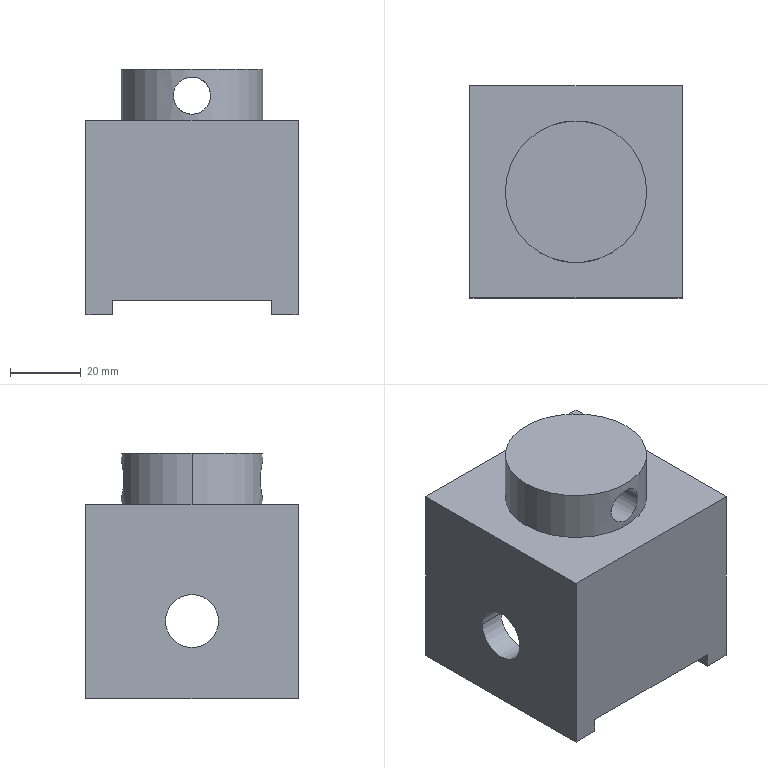Part | NX | features BREP 1 | 1 solid | 23 faces | box 60 x 60 x 69.5 mm | volume 83417 mm3 | plane 15 | cylinder 8 | commonest cylinder face diameters 15 x4 10.5 x2 40 x2
STEP:
#1=CARTESIAN_POINT('',(-5.25,-19.299,7.));
#2=VERTEX_POINT('',#1);
#3=CARTESIAN_POINT('',(5.25,-19.299,7.));
#4=VERTEX_POINT('',#3);
#5=CARTESIAN_POINT('',(-5.25,-19.299,7.));
#6=CARTESIAN_POINT('',(-5.25,-19.299,6.68));
#7=CARTESIAN_POINT('',(-5.203,-19.312,6.178));
#8=CARTESIAN_POINT('',(-5.05,-19.353,5.525));
#9=CARTESIAN_POINT('',(-4.847,-19.404,4.964));
#10=CARTESIAN_POINT('',(-4.714,-19.437,4.682));
#11=CARTESIAN_POINT('',(-4.41,-19.511,4.109));
#12=CARTESIAN_POINT('',(-3.746,-19.654,3.244));
#13=CARTESIAN_POINT('',(-2.935,-19.786,2.621));
#14=CARTESIAN_POINT('',(-2.357,-19.86,2.304));
#15=CARTESIAN_POINT('',(-2.046,-19.896,2.157));
#16=CARTESIAN_POINT('',(-1.491,-19.946,1.955));
#17=CARTESIAN_POINT('',(-0.8306,-19.986,1.798));
#18=CARTESIAN_POINT('',(-0.005315,-20.008,1.718));
#19=CARTESIAN_POINT('',(0.8212,-19.987,1.797));
#20=CARTESIAN_POINT('',(1.478,-19.947,1.951));
#21=CARTESIAN_POINT('',(2.033,-19.898,2.152));
#22=CARTESIAN_POINT('',(2.33,-19.864,2.291));
#23=CARTESIAN_POINT('',(2.909,-19.79,2.605));
#24=CARTESIAN_POINT('',(3.547,-19.687,3.081));
#25=CARTESIAN_POINT('',(4.166,-19.564,3.784));
#26=CARTESIAN_POINT('',(4.479,-19.495,4.243));
#27=CARTESIAN_POINT('',(4.716,-19.437,4.684));
#28=CARTESIAN_POINT('',(4.84,-19.406,4.949));
#29=CARTESIAN_POINT('',(5.049,-19.353,5.522));
#30=CARTESIAN_POINT('',(5.202,-19.312,6.177));
#31=CARTESIAN_POINT('',(5.25,-19.299,6.681));
#32=CARTESIAN_POINT('',(5.25,-19.299,7.));
#33=B_SPLINE_CURVE_WITH_KNOTS('',3,(#5,#6,#7,#8,#9,#10,#11,#12,#13,#14,#15,#16,#17,#18,#19,#20,#21,#22,#23,#24,#25,#26,#27,#28,#29,#30,#31,#32),.UNSPECIFIED.,.F.,.F.,(4,1,1,1,1,1,1,1,1,1,1,1,1,1,1,1,1,1,1,1,1,1,1,1,1,4),(0.,0.0625,0.09375,0.125,0.1562,0.1875,0.25,0.3125,0.3438,0.375,0.4062,0.4375,0.5,0.5625,0.5938,0.625,0.6562,0.6875,0.75,0.7812,0.8125,0.8438,0.875,0.9062,0.9375,1.),.UNSPECIFIED.);
#34=EDGE_CURVE('',#2,#4,#33,.T.);
#35=ORIENTED_EDGE('',*,*,#34,.T.);
#36=CARTESIAN_POINT('',(5.25,19.299,7.));
#37=VERTEX_POINT('',#36);
#38=CARTESIAN_POINT('',(5.25,-19.299,7.));
#39=DIRECTION('',(0.,1.,0.));
#40=VECTOR('',#39,1000.);
#41=LINE('',#38,#40);
#42=EDGE_CURVE('',#37,#4,#41,.F.);
#43=ORIENTED_EDGE('',*,*,#42,.F.);
#44=CARTESIAN_POINT('',(-5.25,19.299,7.));
#45=VERTEX_POINT('',#44);
#46=CARTESIAN_POINT('',(5.25,19.299,7.));
#47=CARTESIAN_POINT('',(5.25,19.299,6.678));
#48=CARTESIAN_POINT('',(5.202,19.313,6.172));
#49=CARTESIAN_POINT('',(5.047,19.354,5.514));
#50=CARTESIAN_POINT('',(4.837,19.406,4.943));
#51=CARTESIAN_POINT('',(4.71,19.439,4.671));
#52=CARTESIAN_POINT('',(4.47,19.497,4.229));
#53=CARTESIAN_POINT('',(4.156,19.566,3.771));
#54=CARTESIAN_POINT('',(3.535,19.69,3.07));
#55=CARTESIAN_POINT('',(2.903,19.791,2.601));
#56=CARTESIAN_POINT('',(2.323,19.865,2.287));
#57=CARTESIAN_POINT('',(2.019,19.9,2.147));
#58=CARTESIAN_POINT('',(1.469,19.948,1.949));
#59=CARTESIAN_POINT('',(0.8131,19.987,1.796));
#60=CARTESIAN_POINT('',(-0.01179,20.009,1.718));
#61=CARTESIAN_POINT('',(-0.8396,19.986,1.8));
#62=CARTESIAN_POINT('',(-1.496,19.946,1.957));
#63=CARTESIAN_POINT('',(-2.051,19.896,2.16));
#64=CARTESIAN_POINT('',(-2.347,19.862,2.299));
#65=CARTESIAN_POINT('',(-2.921,19.788,2.611));
#66=CARTESIAN_POINT('',(-3.746,19.654,3.242));
#67=CARTESIAN_POINT('',(-4.407,19.512,4.104));
#68=CARTESIAN_POINT('',(-4.711,19.438,4.676));
#69=CARTESIAN_POINT('',(-4.842,19.405,4.953));
#70=CARTESIAN_POINT('',(-5.048,19.353,5.518));
#71=CARTESIAN_POINT('',(-5.202,19.312,6.174));
#72=CARTESIAN_POINT('',(-5.25,19.299,6.679));
#73=CARTESIAN_POINT('',(-5.25,19.299,7.));
#74=B_SPLINE_CURVE_WITH_KNOTS('',3,(#46,#47,#48,#49,#50,#51,#52,#53,#54,#55,#56,#57,#58,#59,#60,#61,#62,#63,#64,#65,#66,#67,#68,#69,#70,#71,#72,#73),.UNSPECIFIED.,.F.,.F.,(4,1,1,1,1,1,1,1,1,1,1,1,1,1,1,1,1,1,1,1,1,1,1,1,1,4),(0.,0.0625,0.09375,0.125,0.1562,0.1875,0.2188,0.25,0.3125,0.3438,0.375,0.4062,0.4375,0.5,0.5625,0.5938,0.625,0.6562,0.6875,0.75,0.8125,0.8438,0.875,0.9062,0.9375,1.),.UNSPECIFIED.);
#75=EDGE_CURVE('',#45,#37,#74,.F.);
#76=ORIENTED_EDGE('',*,*,#75,.F.);
#77=CARTESIAN_POINT('',(-5.25,-19.299,7.));
#78=DIRECTION('',(0.,1.,0.));
#79=VECTOR('',#78,1000.);
#80=LINE('',#77,#79);
#81=EDGE_CURVE('',#45,#2,#80,.F.);
#82=ORIENTED_EDGE('',*,*,#81,.T.);
#83=EDGE_LOOP('',(#35,#43,#76,#82));
#84=FACE_BOUND('',#83,.T.);
#85=CARTESIAN_POINT('',(0.,0.,7.));
#86=DIRECTION('',(0.,1.,0.));
#87=DIRECTION('',(-1.,0.,0.));
#88=AXIS2_PLACEMENT_3D('',#85,#86,#87);
#89=CYLINDRICAL_SURFACE('',#88,5.25);
#90=ADVANCED_FACE('',(#84),#89,.F.);
#91=CARTESIAN_POINT('',(5.25,-19.299,7.));
#92=CARTESIAN_POINT('',(5.25,-19.299,7.313));
#93=CARTESIAN_POINT('',(5.204,-19.312,7.811));
#94=CARTESIAN_POINT('',(5.052,-19.353,8.467));
#95=CARTESIAN_POINT('',(4.847,-19.405,9.036));
#96=CARTESIAN_POINT('',(4.712,-19.438,9.323));
#97=CARTESIAN_POINT('',(4.405,-19.512,9.899));
#98=CARTESIAN_POINT('',(3.748,-19.653,10.754));
#99=CARTESIAN_POINT('',(2.936,-19.786,11.379));
#100=CARTESIAN_POINT('',(2.358,-19.86,11.695));
#101=CARTESIAN_POINT('',(2.046,-19.896,11.842));
#102=CARTESIAN_POINT('',(1.494,-19.946,12.044));
#103=CARTESIAN_POINT('',(0.8342,-19.986,12.201));
#104=CARTESIAN_POINT('',(0.006992,-20.009,12.282));
#105=CARTESIAN_POINT('',(-0.8194,-19.987,12.203));
#106=CARTESIAN_POINT('',(-1.476,-19.947,12.049));
#107=CARTESIAN_POINT('',(-2.03,-19.898,11.849));
#108=CARTESIAN_POINT('',(-2.33,-19.863,11.71));
#109=CARTESIAN_POINT('',(-2.91,-19.789,11.394));
#110=CARTESIAN_POINT('',(-3.544,-19.688,10.922));
#111=CARTESIAN_POINT('',(-4.169,-19.563,10.212));
#112=CARTESIAN_POINT('',(-4.482,-19.494,9.752));
#113=CARTESIAN_POINT('',(-4.718,-19.437,9.312));
#114=CARTESIAN_POINT('',(-4.839,-19.406,9.053));
#115=CARTESIAN_POINT('',(-5.049,-19.353,8.48));
#116=CARTESIAN_POINT('',(-5.202,-19.312,7.825));
#117=CARTESIAN_POINT('',(-5.25,-19.299,7.32));
#118=CARTESIAN_POINT('',(-5.25,-19.299,7.));
#119=B_SPLINE_CURVE_WITH_KNOTS('',3,(#91,#92,#93,#94,#95,#96,#97,#98,#99,#100,#101,#102,#103,#104,#105,#106,#107,#108,#109,#110,#111,#112,#113,#114,#115,#116,#117,#118),.UNSPECIFIED.,.F.,.F.,(4,1,1,1,1,1,1,1,1,1,1,1,1,1,1,1,1,1,1,1,1,1,1,1,1,4),(0.,0.0625,0.09375,0.125,0.1562,0.1875,0.25,0.3125,0.3438,0.375,0.4062,0.4375,0.5,0.5625,0.5938,0.625,0.6562,0.6875,0.75,0.7812,0.8125,0.8438,0.875,0.9062,0.9375,1.),.UNSPECIFIED.);
#120=EDGE_CURVE('',#4,#2,#119,.T.);
#121=ORIENTED_EDGE('',*,*,#120,.T.);
#122=ORIENTED_EDGE('',*,*,#81,.F.);
#123=CARTESIAN_POINT('',(-5.25,19.299,7.));
#124=CARTESIAN_POINT('',(-5.25,19.299,7.322));
#125=CARTESIAN_POINT('',(-5.202,19.313,7.828));
#126=CARTESIAN_POINT('',(-5.047,19.354,8.487));
#127=CARTESIAN_POINT('',(-4.838,19.406,9.057));
#128=CARTESIAN_POINT('',(-4.709,19.439,9.33));
#129=CARTESIAN_POINT('',(-4.469,19.497,9.773));
#130=CARTESIAN_POINT('',(-4.154,19.566,10.232));
#131=CARTESIAN_POINT('',(-3.533,19.69,10.931));
#132=CARTESIAN_POINT('',(-2.898,19.792,11.402));
#133=CARTESIAN_POINT('',(-2.316,19.866,11.717));
#134=CARTESIAN_POINT('',(-2.007,19.901,11.858));
#135=CARTESIAN_POINT('',(-1.458,19.949,12.055));
#136=CARTESIAN_POINT('',(-0.8011,19.988,12.206));
#137=CARTESIAN_POINT('',(0.02533,20.009,12.282));
#138=CARTESIAN_POINT('',(0.8493,19.986,12.198));
#139=CARTESIAN_POINT('',(1.504,19.946,12.041));
#140=CARTESIAN_POINT('',(2.057,19.896,11.838));
#141=CARTESIAN_POINT('',(2.353,19.861,11.698));
#142=CARTESIAN_POINT('',(2.925,19.788,11.386));
#143=CARTESIAN_POINT('',(3.75,19.653,10.753));
#144=CARTESIAN_POINT('',(4.408,19.512,9.894));
#145=CARTESIAN_POINT('',(4.713,19.438,9.321));
#146=CARTESIAN_POINT('',(4.844,19.405,9.041));
#147=CARTESIAN_POINT('',(5.05,19.353,8.475));
#148=CARTESIAN_POINT('',(5.203,19.312,7.821));
#149=CARTESIAN_POINT('',(5.25,19.299,7.318));
#150=CARTESIAN_POINT('',(5.25,19.299,7.));
#151=B_SPLINE_CURVE_WITH_KNOTS('',3,(#123,#124,#125,#126,#127,#128,#129,#130,#131,#132,#133,#134,#135,#136,#137,#138,#139,#140,#141,#142,#143,#144,#145,#146,#147,#148,#149,#150),.UNSPECIFIED.,.F.,.F.,(4,1,1,1,1,1,1,1,1,1,1,1,1,1,1,1,1,1,1,1,1,1,1,1,1,4),(0.,0.0625,0.09375,0.125,0.1562,0.1875,0.2188,0.25,0.3125,0.3438,0.375,0.4062,0.4375,0.5,0.5625,0.5938,0.625,0.6562,0.6875,0.75,0.8125,0.8438,0.875,0.9062,0.9375,1.),.UNSPECIFIED.);
#152=EDGE_CURVE('',#37,#45,#151,.F.);
#153=ORIENTED_EDGE('',*,*,#152,.F.);
#154=ORIENTED_EDGE('',*,*,#42,.T.);
#155=EDGE_LOOP('',(#121,#122,#153,#154));
#156=FACE_BOUND('',#155,.T.);
#157=CARTESIAN_POINT('',(0.,0.,7.));
#158=DIRECTION('',(0.,1.,0.));
#159=DIRECTION('',(-1.,0.,0.));
#160=AXIS2_PLACEMENT_3D('',#157,#158,#159);
#161=CYLINDRICAL_SURFACE('',#160,5.25);
#162=ADVANCED_FACE('',(#156),#161,.F.);
#163=CARTESIAN_POINT('',(-20.,0.,0.));
#164=VERTEX_POINT('',#163);
#165=CARTESIAN_POINT('',(20.,0.,0.));
#166=VERTEX_POINT('',#165);
#167=CARTESIAN_POINT('',(0.,0.,0.));
#168=DIRECTION('',(0.,0.,-1.));
#169=DIRECTION('',(-1.,0.,0.));
#170=AXIS2_PLACEMENT_3D('',#167,#168,#169);
#171=CIRCLE('',#170,20.);
#172=EDGE_CURVE('',#164,#166,#171,.T.);
#173=ORIENTED_EDGE('',*,*,#172,.F.);
#174=CARTESIAN_POINT('',(-20.,0.,14.5));
#175=VERTEX_POINT('',#174);
#176=CARTESIAN_POINT('',(-20.,0.,14.5));
#177=DIRECTION('',(0.,0.,-1.));
#178=VECTOR('',#177,1000.);
#179=LINE('',#176,#178);
#180=EDGE_CURVE('',#175,#164,#179,.T.);
#181=ORIENTED_EDGE('',*,*,#180,.F.);
#182=CARTESIAN_POINT('',(20.,0.,14.5));
#183=VERTEX_POINT('',#182);
#184=CARTESIAN_POINT('',(0.,0.,14.5));
#185=DIRECTION('',(0.,0.,1.));
#186=DIRECTION('',(1.,0.,0.));
#187=AXIS2_PLACEMENT_3D('',#184,#185,#186);
#188=CIRCLE('',#187,20.);
#189=EDGE_CURVE('',#183,#175,#188,.T.);
#190=ORIENTED_EDGE('',*,*,#189,.F.);
#191=CARTESIAN_POINT('',(20.,0.,14.5));
#192=DIRECTION('',(0.,0.,-1.));
#193=VECTOR('',#192,1000.);
#194=LINE('',#191,#193);
#195=EDGE_CURVE('',#183,#166,#194,.T.);
#196=ORIENTED_EDGE('',*,*,#195,.T.);
#197=EDGE_LOOP('',(#173,#181,#190,#196));
#198=FACE_BOUND('',#197,.T.);
#199=ORIENTED_EDGE('',*,*,#75,.T.);
#200=ORIENTED_EDGE('',*,*,#152,.T.);
#201=EDGE_LOOP('',(#199,#200));
#202=FACE_BOUND('',#201,.T.);
#203=CARTESIAN_POINT('',(0.,0.,7.25));
#204=DIRECTION('',(0.,0.,1.));
#205=DIRECTION('',(1.,0.,0.));
#206=AXIS2_PLACEMENT_3D('',#203,#204,#205);
#207=CYLINDRICAL_SURFACE('',#206,20.);
#208=ADVANCED_FACE('',(#198,#202),#207,.T.);
#209=CARTESIAN_POINT('',(0.,0.,0.));
#210=DIRECTION('',(0.,0.,-1.));
#211=DIRECTION('',(1.,0.,0.));
#212=AXIS2_PLACEMENT_3D('',#209,#210,#211);
#213=CIRCLE('',#212,20.);
#214=EDGE_CURVE('',#166,#164,#213,.T.);
#215=ORIENTED_EDGE('',*,*,#214,.F.);
#216=ORIENTED_EDGE('',*,*,#195,.F.);
#217=CARTESIAN_POINT('',(0.,0.,14.5));
#218=DIRECTION('',(0.,0.,1.));
#219=DIRECTION('',(-1.,0.,0.));
#220=AXIS2_PLACEMENT_3D('',#217,#218,#219);
#221=CIRCLE('',#220,20.);
#222=EDGE_CURVE('',#175,#183,#221,.T.);
#223=ORIENTED_EDGE('',*,*,#222,.F.);
#224=ORIENTED_EDGE('',*,*,#180,.T.);
#225=EDGE_LOOP('',(#215,#216,#223,#224));
#226=FACE_BOUND('',#225,.T.);
#227=ORIENTED_EDGE('',*,*,#120,.F.);
#228=ORIENTED_EDGE('',*,*,#34,.F.);
#229=EDGE_LOOP('',(#227,#228));
#230=FACE_BOUND('',#229,.T.);
#231=CARTESIAN_POINT('',(0.,0.,7.25));
#232=DIRECTION('',(0.,0.,1.));
#233=DIRECTION('',(1.,0.,0.));
#234=AXIS2_PLACEMENT_3D('',#231,#232,#233);
#235=CYLINDRICAL_SURFACE('',#234,20.);
#236=ADVANCED_FACE('',(#226,#230),#235,.T.);
#237=ORIENTED_EDGE('',*,*,#222,.T.);
#238=ORIENTED_EDGE('',*,*,#189,.T.);
#239=EDGE_LOOP('',(#237,#238));
#240=FACE_BOUND('',#239,.T.);
#241=CARTESIAN_POINT('',(0.,0.,14.5));
#242=DIRECTION('',(0.,0.,1.));
#243=DIRECTION('',(1.,0.,0.));
#244=AXIS2_PLACEMENT_3D('',#241,#242,#243);
#245=PLANE('',#244);
#246=ADVANCED_FACE('',(#240),#245,.T.);
#247=CARTESIAN_POINT('',(30.,-30.,0.));
#248=VERTEX_POINT('',#247);
#249=CARTESIAN_POINT('',(-30.,-30.,0.));
#250=VERTEX_POINT('',#249);
#251=CARTESIAN_POINT('',(30.,-30.,0.));
#252=DIRECTION('',(-1.,0.,0.));
#253=VECTOR('',#252,1000.);
#254=LINE('',#251,#253);
#255=EDGE_CURVE('',#248,#250,#254,.T.);
#256=ORIENTED_EDGE('',*,*,#255,.F.);
#257=CARTESIAN_POINT('',(30.,30.,0.));
#258=VERTEX_POINT('',#257);
#259=CARTESIAN_POINT('',(30.,30.,0.));
#260=DIRECTION('',(0.,-1.,0.));
#261=VECTOR('',#260,1000.);
#262=LINE('',#259,#261);
#263=EDGE_CURVE('',#258,#248,#262,.T.);
#264=ORIENTED_EDGE('',*,*,#263,.F.);
#265=CARTESIAN_POINT('',(-30.,30.,0.));
#266=VERTEX_POINT('',#265);
#267=CARTESIAN_POINT('',(30.,30.,0.));
#268=DIRECTION('',(-1.,0.,0.));
#269=VECTOR('',#268,1000.);
#270=LINE('',#267,#269);
#271=EDGE_CURVE('',#258,#266,#270,.T.);
#272=ORIENTED_EDGE('',*,*,#271,.T.);
#273=CARTESIAN_POINT('',(-30.,30.,0.));
#274=DIRECTION('',(0.,-1.,0.));
#275=VECTOR('',#274,1000.);
#276=LINE('',#273,#275);
#277=EDGE_CURVE('',#266,#250,#276,.T.);
#278=ORIENTED_EDGE('',*,*,#277,.T.);
#279=EDGE_LOOP('',(#256,#264,#272,#278));
#280=FACE_BOUND('',#279,.T.);
#281=ORIENTED_EDGE('',*,*,#172,.T.);
#282=ORIENTED_EDGE('',*,*,#214,.T.);
#283=EDGE_LOOP('',(#281,#282));
#284=FACE_BOUND('',#283,.T.);
#285=CARTESIAN_POINT('',(30.,0.,0.));
#286=DIRECTION('',(0.,0.,-1.));
#287=DIRECTION('',(0.,-1.,0.));
#288=AXIS2_PLACEMENT_3D('',#285,#286,#287);
#289=PLANE('',#288);
#290=ADVANCED_FACE('',(#280,#284),#289,.F.);
#291=CARTESIAN_POINT('',(-30.,-30.,-55.));
#292=VERTEX_POINT('',#291);
#293=CARTESIAN_POINT('',(-30.,-30.,0.));
#294=DIRECTION('',(0.,0.,-1.));
#295=VECTOR('',#294,1000.);
#296=LINE('',#293,#295);
#297=EDGE_CURVE('',#250,#292,#296,.T.);
#298=ORIENTED_EDGE('',*,*,#297,.F.);
#299=ORIENTED_EDGE('',*,*,#277,.F.);
#300=CARTESIAN_POINT('',(-30.,30.,-55.));
#301=VERTEX_POINT('',#300);
#302=CARTESIAN_POINT('',(-30.,30.,0.));
#303=DIRECTION('',(0.,0.,-1.));
#304=VECTOR('',#303,1000.);
#305=LINE('',#302,#304);
#306=EDGE_CURVE('',#266,#301,#305,.T.);
#307=ORIENTED_EDGE('',*,*,#306,.T.);
#308=CARTESIAN_POINT('',(-30.,30.,-55.));
#309=DIRECTION('',(0.,-1.,0.));
#310=VECTOR('',#309,1000.);
#311=LINE('',#308,#310);
#312=EDGE_CURVE('',#301,#292,#311,.T.);
#313=ORIENTED_EDGE('',*,*,#312,.T.);
#314=EDGE_LOOP('',(#298,#299,#307,#313));
#315=FACE_BOUND('',#314,.T.);
#316=CARTESIAN_POINT('',(-30.,-7.5,-33.));
#317=VERTEX_POINT('',#316);
#318=CARTESIAN_POINT('',(-30.,7.5,-33.));
#319=VERTEX_POINT('',#318);
#320=CARTESIAN_POINT('',(-30.,0.,-33.));
#321=DIRECTION('',(1.,0.,0.));
#322=DIRECTION('',(0.,-1.,0.));
#323=AXIS2_PLACEMENT_3D('',#320,#321,#322);
#324=CIRCLE('',#323,7.5);
#325=EDGE_CURVE('',#317,#319,#324,.T.);
#326=ORIENTED_EDGE('',*,*,#325,.T.);
#327=CARTESIAN_POINT('',(-30.,0.,-33.));
#328=DIRECTION('',(1.,0.,0.));
#329=DIRECTION('',(0.,1.,0.));
#330=AXIS2_PLACEMENT_3D('',#327,#328,#329);
#331=CIRCLE('',#330,7.5);
#332=EDGE_CURVE('',#319,#317,#331,.T.);
#333=ORIENTED_EDGE('',*,*,#332,.T.);
#334=EDGE_LOOP('',(#326,#333));
#335=FACE_BOUND('',#334,.T.);
#336=CARTESIAN_POINT('',(-30.,0.,-55.));
#337=DIRECTION('',(-1.,0.,0.));
#338=DIRECTION('',(0.,0.,1.));
#339=AXIS2_PLACEMENT_3D('',#336,#337,#338);
#340=PLANE('',#339);
#341=ADVANCED_FACE('',(#315,#335),#340,.T.);
#342=CARTESIAN_POINT('',(22.5,30.,-55.));
#343=VERTEX_POINT('',#342);
#344=CARTESIAN_POINT('',(30.,30.,-55.));
#345=VERTEX_POINT('',#344);
#346=CARTESIAN_POINT('',(22.5,30.,-55.));
#347=DIRECTION('',(1.,0.,0.));
#348=VECTOR('',#347,1000.);
#349=LINE('',#346,#348);
#350=EDGE_CURVE('',#343,#345,#349,.T.);
#351=ORIENTED_EDGE('',*,*,#350,.T.);
#352=CARTESIAN_POINT('',(30.,-30.,-55.));
#353=VERTEX_POINT('',#352);
#354=CARTESIAN_POINT('',(30.,30.,-55.));
#355=DIRECTION('',(0.,-1.,0.));
#356=VECTOR('',#355,1000.);
#357=LINE('',#354,#356);
#358=EDGE_CURVE('',#345,#353,#357,.T.);
#359=ORIENTED_EDGE('',*,*,#358,.T.);
#360=CARTESIAN_POINT('',(22.5,-30.,-55.));
#361=VERTEX_POINT('',#360);
#362=CARTESIAN_POINT('',(22.5,-30.,-55.));
#363=DIRECTION('',(1.,0.,0.));
#364=VECTOR('',#363,1000.);
#365=LINE('',#362,#364);
#366=EDGE_CURVE('',#361,#353,#365,.T.);
#367=ORIENTED_EDGE('',*,*,#366,.F.);
#368=CARTESIAN_POINT('',(22.5,-30.,-55.));
#369=DIRECTION('',(0.,1.,0.));
#370=VECTOR('',#369,1000.);
#371=LINE('',#368,#370);
#372=EDGE_CURVE('',#361,#343,#371,.T.);
#373=ORIENTED_EDGE('',*,*,#372,.T.);
#374=EDGE_LOOP('',(#351,#359,#367,#373));
#375=FACE_BOUND('',#374,.T.);
#376=CARTESIAN_POINT('',(22.5,0.,-55.));
#377=DIRECTION('',(0.,0.,1.));
#378=DIRECTION('',(1.,0.,0.));
#379=AXIS2_PLACEMENT_3D('',#376,#377,#378);
#380=PLANE('',#379);
#381=ADVANCED_FACE('',(#375),#380,.F.);
#382=CARTESIAN_POINT('',(-22.5,-30.,-55.));
#383=VERTEX_POINT('',#382);
#384=CARTESIAN_POINT('',(-30.,-30.,-55.));
#385=DIRECTION('',(1.,0.,0.));
#386=VECTOR('',#385,1000.);
#387=LINE('',#384,#386);
#388=EDGE_CURVE('',#292,#383,#387,.T.);
#389=ORIENTED_EDGE('',*,*,#388,.F.);
#390=ORIENTED_EDGE('',*,*,#312,.F.);
#391=CARTESIAN_POINT('',(-22.5,30.,-55.));
#392=VERTEX_POINT('',#391);
#393=CARTESIAN_POINT('',(-30.,30.,-55.));
#394=DIRECTION('',(1.,0.,0.));
#395=VECTOR('',#394,1000.);
#396=LINE('',#393,#395);
#397=EDGE_CURVE('',#301,#392,#396,.T.);
#398=ORIENTED_EDGE('',*,*,#397,.T.);
#399=CARTESIAN_POINT('',(-22.5,30.,-55.));
#400=DIRECTION('',(0.,-1.,0.));
#401=VECTOR('',#400,1000.);
#402=LINE('',#399,#401);
#403=EDGE_CURVE('',#392,#383,#402,.T.);
#404=ORIENTED_EDGE('',*,*,#403,.T.);
#405=EDGE_LOOP('',(#389,#390,#398,#404));
#406=FACE_BOUND('',#405,.T.);
#407=CARTESIAN_POINT('',(22.5,0.,-55.));
#408=DIRECTION('',(0.,0.,1.));
#409=DIRECTION('',(1.,0.,0.));
#410=AXIS2_PLACEMENT_3D('',#407,#408,#409);
#411=PLANE('',#410);
#412=ADVANCED_FACE('',(#406),#411,.F.);
#413=CARTESIAN_POINT('',(22.5,28.,-5.));
#414=VERTEX_POINT('',#413);
#415=CARTESIAN_POINT('',(22.5,-28.,-5.));
#416=VERTEX_POINT('',#415);
#417=CARTESIAN_POINT('',(22.5,28.,-5.));
#418=DIRECTION('',(0.,-1.,0.));
#419=VECTOR('',#418,1000.);
#420=LINE('',#417,#419);
#421=EDGE_CURVE('',#414,#416,#420,.T.);
#422=ORIENTED_EDGE('',*,*,#421,.F.);
#423=CARTESIAN_POINT('',(22.5,28.,-51.));
#424=VERTEX_POINT('',#423);
#425=CARTESIAN_POINT('',(22.5,28.,-51.));
#426=DIRECTION('',(0.,0.,1.));
#427=VECTOR('',#426,1000.);
#428=LINE('',#425,#427);
#429=EDGE_CURVE('',#424,#414,#428,.T.);
#430=ORIENTED_EDGE('',*,*,#429,.F.);
#431=CARTESIAN_POINT('',(22.5,30.,-51.));
#432=VERTEX_POINT('',#431);
#433=CARTESIAN_POINT('',(22.5,30.,-51.));
#434=DIRECTION('',(0.,-1.,0.));
#435=VECTOR('',#434,1000.);
#436=LINE('',#433,#435);
#437=EDGE_CURVE('',#432,#424,#436,.T.);
#438=ORIENTED_EDGE('',*,*,#437,.F.);
#439=CARTESIAN_POINT('',(22.5,30.,-55.));
#440=DIRECTION('',(0.,0.,1.));
#441=VECTOR('',#440,1000.);
#442=LINE('',#439,#441);
#443=EDGE_CURVE('',#343,#432,#442,.T.);
#444=ORIENTED_EDGE('',*,*,#443,.F.);
#445=ORIENTED_EDGE('',*,*,#372,.F.);
#446=CARTESIAN_POINT('',(22.5,-30.,-51.));
#447=VERTEX_POINT('',#446);
#448=CARTESIAN_POINT('',(22.5,-30.,-55.));
#449=DIRECTION('',(0.,0.,1.));
#450=VECTOR('',#449,1000.);
#451=LINE('',#448,#450);
#452=EDGE_CURVE('',#361,#447,#451,.T.);
#453=ORIENTED_EDGE('',*,*,#452,.T.);
#454=CARTESIAN_POINT('',(22.5,-28.,-51.));
#455=VERTEX_POINT('',#454);
#456=CARTESIAN_POINT('',(22.5,-28.,-51.));
#457=DIRECTION('',(0.,-1.,0.));
#458=VECTOR('',#457,1000.);
#459=LINE('',#456,#458);
#460=EDGE_CURVE('',#455,#447,#459,.T.);
#461=ORIENTED_EDGE('',*,*,#460,.F.);
#462=CARTESIAN_POINT('',(22.5,-28.,-51.));
#463=DIRECTION('',(0.,0.,1.));
#464=VECTOR('',#463,1000.);
#465=LINE('',#462,#464);
#466=EDGE_CURVE('',#455,#416,#465,.T.);
#467=ORIENTED_EDGE('',*,*,#466,.T.);
#468=EDGE_LOOP('',(#422,#430,#438,#444,#445,#453,#461,#467));
#469=FACE_BOUND('',#468,.T.);
#470=CARTESIAN_POINT('',(22.5,7.5,-33.));
#471=VERTEX_POINT('',#470);
#472=CARTESIAN_POINT('',(22.5,-7.5,-33.));
#473=VERTEX_POINT('',#472);
#474=CARTESIAN_POINT('',(22.5,0.,-33.));
#475=DIRECTION('',(1.,0.,0.));
#476=DIRECTION('',(0.,1.,0.));
#477=AXIS2_PLACEMENT_3D('',#474,#475,#476);
#478=CIRCLE('',#477,7.5);
#479=EDGE_CURVE('',#471,#473,#478,.T.);
#480=ORIENTED_EDGE('',*,*,#479,.T.);
#481=CARTESIAN_POINT('',(22.5,0.,-33.));
#482=DIRECTION('',(1.,0.,0.));
#483=DIRECTION('',(0.,-1.,0.));
#484=AXIS2_PLACEMENT_3D('',#481,#482,#483);
#485=CIRCLE('',#484,7.5);
#486=EDGE_CURVE('',#473,#471,#485,.T.);
#487=ORIENTED_EDGE('',*,*,#486,.T.);
#488=EDGE_LOOP('',(#480,#487));
#489=FACE_BOUND('',#488,.T.);
#490=CARTESIAN_POINT('',(22.5,0.,-5.));
#491=DIRECTION('',(1.,0.,0.));
#492=DIRECTION('',(0.,1.,0.));
#493=AXIS2_PLACEMENT_3D('',#490,#491,#492);
#494=PLANE('',#493);
#495=ADVANCED_FACE('',(#469,#489),#494,.F.);
#496=CARTESIAN_POINT('',(30.,-7.5,-33.));
#497=VERTEX_POINT('',#496);
#498=CARTESIAN_POINT('',(22.5,-7.5,-33.));
#499=DIRECTION('',(1.,0.,0.));
#500=VECTOR('',#499,1000.);
#501=LINE('',#498,#500);
#502=EDGE_CURVE('',#473,#497,#501,.T.);
#503=ORIENTED_EDGE('',*,*,#502,.T.);
#504=CARTESIAN_POINT('',(30.,7.5,-33.));
#505=VERTEX_POINT('',#504);
#506=CARTESIAN_POINT('',(30.,0.,-33.));
#507=DIRECTION('',(-1.,0.,0.));
#508=DIRECTION('',(0.,1.,0.));
#509=AXIS2_PLACEMENT_3D('',#506,#507,#508);
#510=CIRCLE('',#509,7.5);
#511=EDGE_CURVE('',#505,#497,#510,.T.);
#512=ORIENTED_EDGE('',*,*,#511,.F.);
#513=CARTESIAN_POINT('',(22.5,7.5,-33.));
#514=DIRECTION('',(1.,0.,0.));
#515=VECTOR('',#514,1000.);
#516=LINE('',#513,#515);
#517=EDGE_CURVE('',#471,#505,#516,.T.);
#518=ORIENTED_EDGE('',*,*,#517,.F.);
#519=ORIENTED_EDGE('',*,*,#486,.F.);
#520=EDGE_LOOP('',(#503,#512,#518,#519));
#521=FACE_BOUND('',#520,.T.);
#522=CARTESIAN_POINT('',(-0.66,0.,-33.));
#523=DIRECTION('',(1.,0.,0.));
#524=DIRECTION('',(0.,1.,0.));
#525=AXIS2_PLACEMENT_3D('',#522,#523,#524);
#526=CYLINDRICAL_SURFACE('',#525,7.5);
#527=ADVANCED_FACE('',(#521),#526,.F.);
#528=ORIENTED_EDGE('',*,*,#517,.T.);
#529=CARTESIAN_POINT('',(30.,0.,-33.));
#530=DIRECTION('',(-1.,0.,0.));
#531=DIRECTION('',(0.,-1.,0.));
#532=AXIS2_PLACEMENT_3D('',#529,#530,#531);
#533=CIRCLE('',#532,7.5);
#534=EDGE_CURVE('',#497,#505,#533,.T.);
#535=ORIENTED_EDGE('',*,*,#534,.F.);
#536=ORIENTED_EDGE('',*,*,#502,.F.);
#537=ORIENTED_EDGE('',*,*,#479,.F.);
#538=EDGE_LOOP('',(#528,#535,#536,#537));
#539=FACE_BOUND('',#538,.T.);
#540=CARTESIAN_POINT('',(-0.66,0.,-33.));
#541=DIRECTION('',(1.,0.,0.));
#542=DIRECTION('',(0.,1.,0.));
#543=AXIS2_PLACEMENT_3D('',#540,#541,#542);
#544=CYLINDRICAL_SURFACE('',#543,7.5);
#545=ADVANCED_FACE('',(#539),#544,.F.);
#546=CARTESIAN_POINT('',(30.,-30.,-55.));
#547=DIRECTION('',(0.,0.,1.));
#548=VECTOR('',#547,1000.);
#549=LINE('',#546,#548);
#550=EDGE_CURVE('',#353,#248,#549,.T.);
#551=ORIENTED_EDGE('',*,*,#550,.F.);
#552=ORIENTED_EDGE('',*,*,#358,.F.);
#553=CARTESIAN_POINT('',(30.,30.,-55.));
#554=DIRECTION('',(0.,0.,1.));
#555=VECTOR('',#554,1000.);
#556=LINE('',#553,#555);
#557=EDGE_CURVE('',#345,#258,#556,.T.);
#558=ORIENTED_EDGE('',*,*,#557,.T.);
#559=ORIENTED_EDGE('',*,*,#263,.T.);
#560=EDGE_LOOP('',(#551,#552,#558,#559));
#561=FACE_BOUND('',#560,.T.);
#562=ORIENTED_EDGE('',*,*,#511,.T.);
#563=ORIENTED_EDGE('',*,*,#534,.T.);
#564=EDGE_LOOP('',(#562,#563));
#565=FACE_BOUND('',#564,.T.);
#566=CARTESIAN_POINT('',(30.,0.,0.));
#567=DIRECTION('',(1.,0.,0.));
#568=DIRECTION('',(0.,1.,0.));
#569=AXIS2_PLACEMENT_3D('',#566,#567,#568);
#570=PLANE('',#569);
#571=ADVANCED_FACE('',(#561,#565),#570,.T.);
#572=CARTESIAN_POINT('',(-22.5,30.,-51.));
#573=VERTEX_POINT('',#572);
#574=CARTESIAN_POINT('',(-22.5,30.,-55.));
#575=DIRECTION('',(0.,0.,1.));
#576=VECTOR('',#575,1000.);
#577=LINE('',#574,#576);
#578=EDGE_CURVE('',#392,#573,#577,.T.);
#579=ORIENTED_EDGE('',*,*,#578,.F.);
#580=ORIENTED_EDGE('',*,*,#397,.F.);
#581=ORIENTED_EDGE('',*,*,#306,.F.);
#582=ORIENTED_EDGE('',*,*,#271,.F.);
#583=ORIENTED_EDGE('',*,*,#557,.F.);
#584=ORIENTED_EDGE('',*,*,#350,.F.);
#585=ORIENTED_EDGE('',*,*,#443,.T.);
#586=CARTESIAN_POINT('',(22.5,30.,-51.));
#587=DIRECTION('',(-1.,0.,0.));
#588=VECTOR('',#587,1000.);
#589=LINE('',#586,#588);
#590=EDGE_CURVE('',#432,#573,#589,.T.);
#591=ORIENTED_EDGE('',*,*,#590,.T.);
#592=EDGE_LOOP('',(#579,#580,#581,#582,#583,#584,#585,#591));
#593=FACE_BOUND('',#592,.T.);
#594=CARTESIAN_POINT('',(0.,30.,0.));
#595=DIRECTION('',(0.,1.,0.));
#596=DIRECTION('',(1.,0.,0.));
#597=AXIS2_PLACEMENT_3D('',#594,#595,#596);
#598=PLANE('',#597);
#599=ADVANCED_FACE('',(#593),#598,.T.);
#600=CARTESIAN_POINT('',(-22.5,-30.,-51.));
#601=VERTEX_POINT('',#600);
#602=CARTESIAN_POINT('',(-22.5,-28.,-51.));
#603=VERTEX_POINT('',#602);
#604=CARTESIAN_POINT('',(-22.5,-30.,-51.));
#605=DIRECTION('',(0.,1.,0.));
#606=VECTOR('',#605,1000.);
#607=LINE('',#604,#606);
#608=EDGE_CURVE('',#601,#603,#607,.T.);
#609=ORIENTED_EDGE('',*,*,#608,.T.);
#610=CARTESIAN_POINT('',(22.5,-28.,-51.));
#611=DIRECTION('',(-1.,0.,0.));
#612=VECTOR('',#611,1000.);
#613=LINE('',#610,#612);
#614=EDGE_CURVE('',#455,#603,#613,.T.);
#615=ORIENTED_EDGE('',*,*,#614,.F.);
#616=ORIENTED_EDGE('',*,*,#460,.T.);
#617=CARTESIAN_POINT('',(22.5,-30.,-51.));
#618=DIRECTION('',(-1.,0.,0.));
#619=VECTOR('',#618,1000.);
#620=LINE('',#617,#619);
#621=EDGE_CURVE('',#447,#601,#620,.T.);
#622=ORIENTED_EDGE('',*,*,#621,.T.);
#623=EDGE_LOOP('',(#609,#615,#616,#622));
#624=FACE_BOUND('',#623,.T.);
#625=CARTESIAN_POINT('',(0.,0.,-51.));
#626=DIRECTION('',(0.,0.,-1.));
#627=DIRECTION('',(0.,-1.,0.));
#628=AXIS2_PLACEMENT_3D('',#625,#626,#627);
#629=PLANE('',#628);
#630=ADVANCED_FACE('',(#624),#629,.T.);
#631=CARTESIAN_POINT('',(-22.5,28.,-51.));
#632=VERTEX_POINT('',#631);
#633=CARTESIAN_POINT('',(-22.5,28.,-51.));
#634=DIRECTION('',(0.,1.,0.));
#635=VECTOR('',#634,1000.);
#636=LINE('',#633,#635);
#637=EDGE_CURVE('',#632,#573,#636,.T.);
#638=ORIENTED_EDGE('',*,*,#637,.T.);
#639=ORIENTED_EDGE('',*,*,#590,.F.);
#640=ORIENTED_EDGE('',*,*,#437,.T.);
#641=CARTESIAN_POINT('',(22.5,28.,-51.));
#642=DIRECTION('',(-1.,0.,0.));
#643=VECTOR('',#642,1000.);
#644=LINE('',#641,#643);
#645=EDGE_CURVE('',#424,#632,#644,.T.);
#646=ORIENTED_EDGE('',*,*,#645,.T.);
#647=EDGE_LOOP('',(#638,#639,#640,#646));
#648=FACE_BOUND('',#647,.T.);
#649=CARTESIAN_POINT('',(0.,0.,-51.));
#650=DIRECTION('',(0.,0.,-1.));
#651=DIRECTION('',(0.,-1.,0.));
#652=AXIS2_PLACEMENT_3D('',#649,#650,#651);
#653=PLANE('',#652);
#654=ADVANCED_FACE('',(#648),#653,.T.);
#655=ORIENTED_EDGE('',*,*,#452,.F.);
#656=ORIENTED_EDGE('',*,*,#366,.T.);
#657=ORIENTED_EDGE('',*,*,#550,.T.);
#658=ORIENTED_EDGE('',*,*,#255,.T.);
#659=ORIENTED_EDGE('',*,*,#297,.T.);
#660=ORIENTED_EDGE('',*,*,#388,.T.);
#661=CARTESIAN_POINT('',(-22.5,-30.,-55.));
#662=DIRECTION('',(0.,0.,1.));
#663=VECTOR('',#662,1000.);
#664=LINE('',#661,#663);
#665=EDGE_CURVE('',#383,#601,#664,.T.);
#666=ORIENTED_EDGE('',*,*,#665,.T.);
#667=ORIENTED_EDGE('',*,*,#621,.F.);
#668=EDGE_LOOP('',(#655,#656,#657,#658,#659,#660,#666,#667));
#669=FACE_BOUND('',#668,.T.);
#670=CARTESIAN_POINT('',(0.,-30.,0.));
#671=DIRECTION('',(0.,1.,0.));
#672=DIRECTION('',(1.,0.,0.));
#673=AXIS2_PLACEMENT_3D('',#670,#671,#672);
#674=PLANE('',#673);
#675=ADVANCED_FACE('',(#669),#674,.F.);
#676=ORIENTED_EDGE('',*,*,#578,.T.);
#677=ORIENTED_EDGE('',*,*,#637,.F.);
#678=CARTESIAN_POINT('',(-22.5,28.,-5.));
#679=VERTEX_POINT('',#678);
#680=CARTESIAN_POINT('',(-22.5,28.,-51.));
#681=DIRECTION('',(0.,0.,1.));
#682=VECTOR('',#681,1000.);
#683=LINE('',#680,#682);
#684=EDGE_CURVE('',#632,#679,#683,.T.);
#685=ORIENTED_EDGE('',*,*,#684,.T.);
#686=CARTESIAN_POINT('',(-22.5,-28.,-5.));
#687=VERTEX_POINT('',#686);
#688=CARTESIAN_POINT('',(-22.5,28.,-5.));
#689=DIRECTION('',(0.,-1.,0.));
#690=VECTOR('',#689,1000.);
#691=LINE('',#688,#690);
#692=EDGE_CURVE('',#679,#687,#691,.T.);
#693=ORIENTED_EDGE('',*,*,#692,.T.);
#694=CARTESIAN_POINT('',(-22.5,-28.,-51.));
#695=DIRECTION('',(0.,0.,1.));
#696=VECTOR('',#695,1000.);
#697=LINE('',#694,#696);
#698=EDGE_CURVE('',#603,#687,#697,.T.);
#699=ORIENTED_EDGE('',*,*,#698,.F.);
#700=ORIENTED_EDGE('',*,*,#608,.F.);
#701=ORIENTED_EDGE('',*,*,#665,.F.);
#702=ORIENTED_EDGE('',*,*,#403,.F.);
#703=EDGE_LOOP('',(#676,#677,#685,#693,#699,#700,#701,#702));
#704=FACE_BOUND('',#703,.T.);
#705=CARTESIAN_POINT('',(-22.5,-7.5,-33.));
#706=VERTEX_POINT('',#705);
#707=CARTESIAN_POINT('',(-22.5,7.5,-33.));
#708=VERTEX_POINT('',#707);
#709=CARTESIAN_POINT('',(-22.5,0.,-33.));
#710=DIRECTION('',(-1.,0.,0.));
#711=DIRECTION('',(0.,-1.,0.));
#712=AXIS2_PLACEMENT_3D('',#709,#710,#711);
#713=CIRCLE('',#712,7.5);
#714=EDGE_CURVE('',#706,#708,#713,.T.);
#715=ORIENTED_EDGE('',*,*,#714,.T.);
#716=CARTESIAN_POINT('',(-22.5,0.,-33.));
#717=DIRECTION('',(-1.,0.,0.));
#718=DIRECTION('',(0.,1.,0.));
#719=AXIS2_PLACEMENT_3D('',#716,#717,#718);
#720=CIRCLE('',#719,7.5);
#721=EDGE_CURVE('',#708,#706,#720,.T.);
#722=ORIENTED_EDGE('',*,*,#721,.T.);
#723=EDGE_LOOP('',(#715,#722));
#724=FACE_BOUND('',#723,.T.);
#725=CARTESIAN_POINT('',(-22.5,0.,-55.));
#726=DIRECTION('',(-1.,0.,0.));
#727=DIRECTION('',(0.,0.,1.));
#728=AXIS2_PLACEMENT_3D('',#725,#726,#727);
#729=PLANE('',#728);
#730=ADVANCED_FACE('',(#704,#724),#729,.F.);
#731=ORIENTED_EDGE('',*,*,#325,.F.);
#732=CARTESIAN_POINT('',(-30.,-7.5,-33.));
#733=DIRECTION('',(1.,0.,0.));
#734=VECTOR('',#733,1000.);
#735=LINE('',#732,#734);
#736=EDGE_CURVE('',#317,#706,#735,.T.);
#737=ORIENTED_EDGE('',*,*,#736,.T.);
#738=ORIENTED_EDGE('',*,*,#721,.F.);
#739=CARTESIAN_POINT('',(-30.,7.5,-33.));
#740=DIRECTION('',(1.,0.,0.));
#741=VECTOR('',#740,1000.);
#742=LINE('',#739,#741);
#743=EDGE_CURVE('',#319,#708,#742,.T.);
#744=ORIENTED_EDGE('',*,*,#743,.F.);
#745=EDGE_LOOP('',(#731,#737,#738,#744));
#746=FACE_BOUND('',#745,.T.);
#747=CARTESIAN_POINT('',(-0.66,0.,-33.));
#748=DIRECTION('',(1.,0.,0.));
#749=DIRECTION('',(0.,1.,0.));
#750=AXIS2_PLACEMENT_3D('',#747,#748,#749);
#751=CYLINDRICAL_SURFACE('',#750,7.5);
#752=ADVANCED_FACE('',(#746),#751,.F.);
#753=ORIENTED_EDGE('',*,*,#332,.F.);
#754=ORIENTED_EDGE('',*,*,#743,.T.);
#755=ORIENTED_EDGE('',*,*,#714,.F.);
#756=ORIENTED_EDGE('',*,*,#736,.F.);
#757=EDGE_LOOP('',(#753,#754,#755,#756));
#758=FACE_BOUND('',#757,.T.);
#759=CARTESIAN_POINT('',(-0.66,0.,-33.));
#760=DIRECTION('',(1.,0.,0.));
#761=DIRECTION('',(0.,1.,0.));
#762=AXIS2_PLACEMENT_3D('',#759,#760,#761);
#763=CYLINDRICAL_SURFACE('',#762,7.5);
#764=ADVANCED_FACE('',(#758),#763,.F.);
#765=ORIENTED_EDGE('',*,*,#698,.T.);
#766=CARTESIAN_POINT('',(22.5,-28.,-5.));
#767=DIRECTION('',(-1.,0.,0.));
#768=VECTOR('',#767,1000.);
#769=LINE('',#766,#768);
#770=EDGE_CURVE('',#416,#687,#769,.T.);
#771=ORIENTED_EDGE('',*,*,#770,.F.);
#772=ORIENTED_EDGE('',*,*,#466,.F.);
#773=ORIENTED_EDGE('',*,*,#614,.T.);
#774=EDGE_LOOP('',(#765,#771,#772,#773));
#775=FACE_BOUND('',#774,.T.);
#776=CARTESIAN_POINT('',(22.5,-28.,-5.));
#777=DIRECTION('',(0.,-1.,0.));
#778=DIRECTION('',(0.,0.,-1.));
#779=AXIS2_PLACEMENT_3D('',#776,#777,#778);
#780=PLANE('',#779);
#781=ADVANCED_FACE('',(#775),#780,.F.);
#782=ORIENTED_EDGE('',*,*,#692,.F.);
#783=CARTESIAN_POINT('',(-22.5,28.,-5.));
#784=DIRECTION('',(1.,0.,0.));
#785=VECTOR('',#784,1000.);
#786=LINE('',#783,#785);
#787=EDGE_CURVE('',#679,#414,#786,.T.);
#788=ORIENTED_EDGE('',*,*,#787,.T.);
#789=ORIENTED_EDGE('',*,*,#421,.T.);
#790=ORIENTED_EDGE('',*,*,#770,.T.);
#791=EDGE_LOOP('',(#782,#788,#789,#790));
#792=FACE_BOUND('',#791,.T.);
#793=CARTESIAN_POINT('',(22.5,0.,-5.));
#794=DIRECTION('',(0.,0.,-1.));
#795=DIRECTION('',(0.,-1.,0.));
#796=AXIS2_PLACEMENT_3D('',#793,#794,#795);
#797=PLANE('',#796);
#798=ADVANCED_FACE('',(#792),#797,.T.);
#799=ORIENTED_EDGE('',*,*,#429,.T.);
#800=ORIENTED_EDGE('',*,*,#787,.F.);
#801=ORIENTED_EDGE('',*,*,#684,.F.);
#802=ORIENTED_EDGE('',*,*,#645,.F.);
#803=EDGE_LOOP('',(#799,#800,#801,#802));
#804=FACE_BOUND('',#803,.T.);
#805=CARTESIAN_POINT('',(22.5,28.,-5.));
#806=DIRECTION('',(0.,-1.,0.));
#807=DIRECTION('',(0.,0.,-1.));
#808=AXIS2_PLACEMENT_3D('',#805,#806,#807);
#809=PLANE('',#808);
#810=ADVANCED_FACE('',(#804),#809,.T.);
#811=CLOSED_SHELL('',(#90,#162,#208,#236,#246,#290,#341,#381,#412,#495,#527,#545,#571,#599,#630,#654,#675,#730,#752,#764,#781,#798,#810));
#812=MANIFOLD_SOLID_BREP('',#811);
#813=(LENGTH_UNIT()NAMED_UNIT(*)SI_UNIT(.MILLI.,.METRE.));
#814=UNCERTAINTY_MEASURE_WITH_UNIT(LENGTH_MEASURE(0.0508),#813,'','');
#815=(NAMED_UNIT(*)PLANE_ANGLE_UNIT()SI_UNIT($,.RADIAN.));
#816=(NAMED_UNIT(*)SI_UNIT($,.STERADIAN.)SOLID_ANGLE_UNIT());
#817=(GEOMETRIC_REPRESENTATION_CONTEXT(3)GLOBAL_UNCERTAINTY_ASSIGNED_CONTEXT((#814))GLOBAL_UNIT_ASSIGNED_CONTEXT((#813,#815,#816))REPRESENTATION_CONTEXT('',''));
#818=ADVANCED_BREP_SHAPE_REPRESENTATION('',(#812),#817);